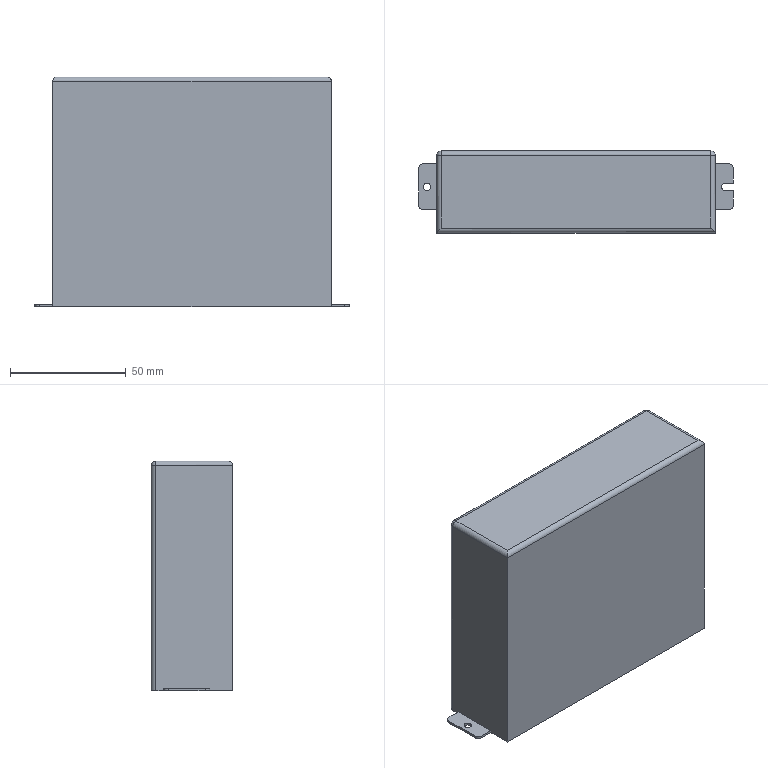Part | NX | features BREP 1 | 1 solid | 31 faces | box 136 x 35.4 x 99.5 mm | volume 424636 mm3 | plane 17 | cylinder 12 | sphere 2 | commonest cylinder face diameters 4 x10 3.2 x2
STEP:
#1=CARTESIAN_POINT('',(-66.1,2.3,0.));
#2=VERTEX_POINT('',#1);
#3=CARTESIAN_POINT('',(-64.5,2.3,0.));
#4=DIRECTION('',(0.,0.,-1.));
#5=DIRECTION('',(-1.,0.,0.));
#6=AXIS2_PLACEMENT_3D('',#3,#4,#5);
#7=CIRCLE('',#6,1.6);
#8=EDGE_CURVE('',#2,#2,#7,.T.);
#9=ORIENTED_EDGE('',*,*,#8,.T.);
#10=EDGE_LOOP('',(#9));
#11=FACE_BOUND('',#10,.T.);
#12=CARTESIAN_POINT('',(-66.1,2.3,1.));
#13=VERTEX_POINT('',#12);
#14=CARTESIAN_POINT('',(-64.5,2.3,1.));
#15=DIRECTION('',(0.,0.,-1.));
#16=DIRECTION('',(-1.,0.,0.));
#17=AXIS2_PLACEMENT_3D('',#14,#15,#16);
#18=CIRCLE('',#17,1.6);
#19=EDGE_CURVE('',#13,#13,#18,.T.);
#20=ORIENTED_EDGE('',*,*,#19,.F.);
#21=EDGE_LOOP('',(#20));
#22=FACE_BOUND('',#21,.T.);
#23=CARTESIAN_POINT('',(-64.5,2.3,10.));
#24=DIRECTION('',(0.,0.,-1.));
#25=DIRECTION('',(-1.,0.,0.));
#26=AXIS2_PLACEMENT_3D('',#23,#24,#25);
#27=CYLINDRICAL_SURFACE('',#26,1.6);
#28=ADVANCED_FACE('',(#11,#22),#27,.F.);
#29=CARTESIAN_POINT('',(64.5,3.9,1.));
#30=VERTEX_POINT('',#29);
#31=CARTESIAN_POINT('',(64.5,0.7,1.));
#32=VERTEX_POINT('',#31);
#33=CARTESIAN_POINT('',(64.5,2.3,1.));
#34=DIRECTION('',(0.,0.,1.));
#35=DIRECTION('',(1.,0.,0.));
#36=AXIS2_PLACEMENT_3D('',#33,#34,#35);
#37=CIRCLE('',#36,1.6);
#38=EDGE_CURVE('',#30,#32,#37,.T.);
#39=ORIENTED_EDGE('',*,*,#38,.T.);
#40=CARTESIAN_POINT('',(64.5,0.7,0.));
#41=VERTEX_POINT('',#40);
#42=CARTESIAN_POINT('',(64.5,0.7,10.));
#43=DIRECTION('',(0.,0.,-1.));
#44=VECTOR('',#43,1000.);
#45=LINE('',#42,#44);
#46=EDGE_CURVE('',#32,#41,#45,.T.);
#47=ORIENTED_EDGE('',*,*,#46,.T.);
#48=CARTESIAN_POINT('',(64.5,3.9,0.));
#49=VERTEX_POINT('',#48);
#50=CARTESIAN_POINT('',(64.5,2.3,0.));
#51=DIRECTION('',(0.,0.,-1.));
#52=DIRECTION('',(-1.,0.,0.));
#53=AXIS2_PLACEMENT_3D('',#50,#51,#52);
#54=CIRCLE('',#53,1.6);
#55=EDGE_CURVE('',#41,#49,#54,.T.);
#56=ORIENTED_EDGE('',*,*,#55,.T.);
#57=CARTESIAN_POINT('',(64.5,3.9,10.));
#58=DIRECTION('',(0.,0.,-1.));
#59=VECTOR('',#58,1000.);
#60=LINE('',#57,#59);
#61=EDGE_CURVE('',#30,#49,#60,.T.);
#62=ORIENTED_EDGE('',*,*,#61,.F.);
#63=EDGE_LOOP('',(#39,#47,#56,#62));
#64=FACE_BOUND('',#63,.T.);
#65=CARTESIAN_POINT('',(64.5,2.3,10.));
#66=DIRECTION('',(0.,0.,-1.));
#67=DIRECTION('',(-1.,0.,0.));
#68=AXIS2_PLACEMENT_3D('',#65,#66,#67);
#69=CYLINDRICAL_SURFACE('',#68,1.6);
#70=ADVANCED_FACE('',(#64),#69,.F.);
#71=CARTESIAN_POINT('',(68.,0.7,1.));
#72=VERTEX_POINT('',#71);
#73=CARTESIAN_POINT('',(68.,0.7,0.));
#74=VERTEX_POINT('',#73);
#75=CARTESIAN_POINT('',(68.,0.7,10.));
#76=DIRECTION('',(0.,0.,-1.));
#77=VECTOR('',#76,1000.);
#78=LINE('',#75,#77);
#79=EDGE_CURVE('',#72,#74,#78,.T.);
#80=ORIENTED_EDGE('',*,*,#79,.F.);
#81=CARTESIAN_POINT('',(68.,-5.7,1.));
#82=VERTEX_POINT('',#81);
#83=CARTESIAN_POINT('',(68.,0.05,1.));
#84=DIRECTION('',(0.,-1.,0.));
#85=VECTOR('',#84,1000.);
#86=LINE('',#83,#85);
#87=EDGE_CURVE('',#72,#82,#86,.T.);
#88=ORIENTED_EDGE('',*,*,#87,.T.);
#89=CARTESIAN_POINT('',(68.,-5.7,0.));
#90=VERTEX_POINT('',#89);
#91=CARTESIAN_POINT('',(68.,-5.7,1.));
#92=DIRECTION('',(0.,0.,-1.));
#93=VECTOR('',#92,1000.);
#94=LINE('',#91,#93);
#95=EDGE_CURVE('',#82,#90,#94,.T.);
#96=ORIENTED_EDGE('',*,*,#95,.T.);
#97=CARTESIAN_POINT('',(68.,10.3,0.));
#98=DIRECTION('',(0.,-1.,0.));
#99=VECTOR('',#98,1000.);
#100=LINE('',#97,#99);
#101=EDGE_CURVE('',#74,#90,#100,.T.);
#102=ORIENTED_EDGE('',*,*,#101,.F.);
#103=EDGE_LOOP('',(#80,#88,#96,#102));
#104=FACE_BOUND('',#103,.T.);
#105=CARTESIAN_POINT('',(68.,0.05,1.));
#106=DIRECTION('',(1.,0.,0.));
#107=DIRECTION('',(0.,1.,0.));
#108=AXIS2_PLACEMENT_3D('',#105,#106,#107);
#109=PLANE('',#108);
#110=ADVANCED_FACE('',(#104),#109,.T.);
#111=ORIENTED_EDGE('',*,*,#19,.T.);
#112=EDGE_LOOP('',(#111));
#113=FACE_BOUND('',#112,.T.);
#114=CARTESIAN_POINT('',(-68.,10.3,1.));
#115=VERTEX_POINT('',#114);
#116=CARTESIAN_POINT('',(-66.,12.3,1.));
#117=VERTEX_POINT('',#116);
#118=CARTESIAN_POINT('',(-66.,10.3,1.));
#119=DIRECTION('',(0.,0.,-1.));
#120=DIRECTION('',(-1.,0.,0.));
#121=AXIS2_PLACEMENT_3D('',#118,#119,#120);
#122=CIRCLE('',#121,2.);
#123=EDGE_CURVE('',#115,#117,#122,.T.);
#124=ORIENTED_EDGE('',*,*,#123,.F.);
#125=CARTESIAN_POINT('',(-68.,-5.7,1.));
#126=VERTEX_POINT('',#125);
#127=CARTESIAN_POINT('',(-68.,-1.725,1.));
#128=DIRECTION('',(0.,1.,0.));
#129=VECTOR('',#128,1000.);
#130=LINE('',#127,#129);
#131=EDGE_CURVE('',#126,#115,#130,.T.);
#132=ORIENTED_EDGE('',*,*,#131,.F.);
#133=CARTESIAN_POINT('',(-66.,-7.7,1.));
#134=VERTEX_POINT('',#133);
#135=CARTESIAN_POINT('',(-66.,-5.7,1.));
#136=DIRECTION('',(0.,0.,-1.));
#137=DIRECTION('',(-1.,0.,0.));
#138=AXIS2_PLACEMENT_3D('',#135,#136,#137);
#139=CIRCLE('',#138,2.);
#140=EDGE_CURVE('',#134,#126,#139,.T.);
#141=ORIENTED_EDGE('',*,*,#140,.F.);
#142=CARTESIAN_POINT('',(-60.3,-7.7,1.));
#143=VERTEX_POINT('',#142);
#144=CARTESIAN_POINT('',(-66.,-7.7,1.));
#145=DIRECTION('',(-1.,0.,0.));
#146=VECTOR('',#145,1000.);
#147=LINE('',#144,#146);
#148=EDGE_CURVE('',#143,#134,#147,.T.);
#149=ORIENTED_EDGE('',*,*,#148,.F.);
#150=CARTESIAN_POINT('',(-60.3,12.3,1.));
#151=VERTEX_POINT('',#150);
#152=CARTESIAN_POINT('',(-60.3,12.3,1.));
#153=DIRECTION('',(0.,-1.,0.));
#154=VECTOR('',#153,1000.);
#155=LINE('',#152,#154);
#156=EDGE_CURVE('',#151,#143,#155,.T.);
#157=ORIENTED_EDGE('',*,*,#156,.F.);
#158=CARTESIAN_POINT('',(-60.3,12.3,1.));
#159=DIRECTION('',(1.,0.,0.));
#160=VECTOR('',#159,1000.);
#161=LINE('',#158,#160);
#162=EDGE_CURVE('',#117,#151,#161,.T.);
#163=ORIENTED_EDGE('',*,*,#162,.F.);
#164=EDGE_LOOP('',(#124,#132,#141,#149,#157,#163));
#165=FACE_BOUND('',#164,.T.);
#166=CARTESIAN_POINT('',(-66.,10.3,1.));
#167=DIRECTION('',(0.,0.,-1.));
#168=DIRECTION('',(0.,-1.,0.));
#169=AXIS2_PLACEMENT_3D('',#166,#167,#168);
#170=PLANE('',#169);
#171=ADVANCED_FACE('',(#113,#165),#170,.F.);
#172=CARTESIAN_POINT('',(-66.,12.3,0.));
#173=VERTEX_POINT('',#172);
#174=CARTESIAN_POINT('',(-60.3,12.3,0.));
#175=VERTEX_POINT('',#174);
#176=CARTESIAN_POINT('',(-60.3,12.3,0.));
#177=DIRECTION('',(1.,0.,0.));
#178=VECTOR('',#177,1000.);
#179=LINE('',#176,#178);
#180=EDGE_CURVE('',#173,#175,#179,.T.);
#181=ORIENTED_EDGE('',*,*,#180,.F.);
#182=CARTESIAN_POINT('',(-66.,12.3,1.));
#183=DIRECTION('',(0.,0.,-1.));
#184=VECTOR('',#183,1000.);
#185=LINE('',#182,#184);
#186=EDGE_CURVE('',#117,#173,#185,.T.);
#187=ORIENTED_EDGE('',*,*,#186,.F.);
#188=ORIENTED_EDGE('',*,*,#162,.T.);
#189=CARTESIAN_POINT('',(-60.3,12.3,1.));
#190=DIRECTION('',(0.,0.,-1.));
#191=VECTOR('',#190,1000.);
#192=LINE('',#189,#191);
#193=EDGE_CURVE('',#151,#175,#192,.T.);
#194=ORIENTED_EDGE('',*,*,#193,.T.);
#195=EDGE_LOOP('',(#181,#187,#188,#194));
#196=FACE_BOUND('',#195,.T.);
#197=CARTESIAN_POINT('',(-60.3,12.3,1.));
#198=DIRECTION('',(0.,1.,0.));
#199=DIRECTION('',(1.,0.,0.));
#200=AXIS2_PLACEMENT_3D('',#197,#198,#199);
#201=PLANE('',#200);
#202=ADVANCED_FACE('',(#196),#201,.T.);
#203=CARTESIAN_POINT('',(-60.3,-7.7,0.));
#204=VERTEX_POINT('',#203);
#205=CARTESIAN_POINT('',(-66.,-7.7,0.));
#206=VERTEX_POINT('',#205);
#207=CARTESIAN_POINT('',(-66.,-7.7,0.));
#208=DIRECTION('',(-1.,0.,0.));
#209=VECTOR('',#208,1000.);
#210=LINE('',#207,#209);
#211=EDGE_CURVE('',#204,#206,#210,.T.);
#212=ORIENTED_EDGE('',*,*,#211,.F.);
#213=CARTESIAN_POINT('',(-60.3,-7.7,1.));
#214=DIRECTION('',(0.,0.,-1.));
#215=VECTOR('',#214,1000.);
#216=LINE('',#213,#215);
#217=EDGE_CURVE('',#143,#204,#216,.T.);
#218=ORIENTED_EDGE('',*,*,#217,.F.);
#219=ORIENTED_EDGE('',*,*,#148,.T.);
#220=CARTESIAN_POINT('',(-66.,-7.7,1.));
#221=DIRECTION('',(0.,0.,-1.));
#222=VECTOR('',#221,1000.);
#223=LINE('',#220,#222);
#224=EDGE_CURVE('',#134,#206,#223,.T.);
#225=ORIENTED_EDGE('',*,*,#224,.T.);
#226=EDGE_LOOP('',(#212,#218,#219,#225));
#227=FACE_BOUND('',#226,.T.);
#228=CARTESIAN_POINT('',(-66.,-7.7,1.));
#229=DIRECTION('',(0.,-1.,0.));
#230=DIRECTION('',(0.,0.,-1.));
#231=AXIS2_PLACEMENT_3D('',#228,#229,#230);
#232=PLANE('',#231);
#233=ADVANCED_FACE('',(#227),#232,.T.);
#234=CARTESIAN_POINT('',(-68.,-5.7,0.));
#235=VERTEX_POINT('',#234);
#236=CARTESIAN_POINT('',(-66.,-5.7,0.));
#237=DIRECTION('',(0.,0.,-1.));
#238=DIRECTION('',(-1.,0.,0.));
#239=AXIS2_PLACEMENT_3D('',#236,#237,#238);
#240=CIRCLE('',#239,2.);
#241=EDGE_CURVE('',#206,#235,#240,.T.);
#242=ORIENTED_EDGE('',*,*,#241,.F.);
#243=ORIENTED_EDGE('',*,*,#224,.F.);
#244=ORIENTED_EDGE('',*,*,#140,.T.);
#245=CARTESIAN_POINT('',(-68.,-5.7,1.));
#246=DIRECTION('',(0.,0.,-1.));
#247=VECTOR('',#246,1000.);
#248=LINE('',#245,#247);
#249=EDGE_CURVE('',#126,#235,#248,.T.);
#250=ORIENTED_EDGE('',*,*,#249,.T.);
#251=EDGE_LOOP('',(#242,#243,#244,#250));
#252=FACE_BOUND('',#251,.T.);
#253=CARTESIAN_POINT('',(-66.,-5.7,1.));
#254=DIRECTION('',(0.,0.,-1.));
#255=DIRECTION('',(-1.,0.,0.));
#256=AXIS2_PLACEMENT_3D('',#253,#254,#255);
#257=CYLINDRICAL_SURFACE('',#256,2.);
#258=ADVANCED_FACE('',(#252),#257,.T.);
#259=CARTESIAN_POINT('',(-68.,10.3,0.));
#260=VERTEX_POINT('',#259);
#261=CARTESIAN_POINT('',(-68.,10.3,0.));
#262=DIRECTION('',(0.,1.,0.));
#263=VECTOR('',#262,1000.);
#264=LINE('',#261,#263);
#265=EDGE_CURVE('',#235,#260,#264,.T.);
#266=ORIENTED_EDGE('',*,*,#265,.F.);
#267=ORIENTED_EDGE('',*,*,#249,.F.);
#268=ORIENTED_EDGE('',*,*,#131,.T.);
#269=CARTESIAN_POINT('',(-68.,10.3,1.));
#270=DIRECTION('',(0.,0.,-1.));
#271=VECTOR('',#270,1000.);
#272=LINE('',#269,#271);
#273=EDGE_CURVE('',#115,#260,#272,.T.);
#274=ORIENTED_EDGE('',*,*,#273,.T.);
#275=EDGE_LOOP('',(#266,#267,#268,#274));
#276=FACE_BOUND('',#275,.T.);
#277=CARTESIAN_POINT('',(-68.,10.3,1.));
#278=DIRECTION('',(-1.,0.,0.));
#279=DIRECTION('',(0.,0.,1.));
#280=AXIS2_PLACEMENT_3D('',#277,#278,#279);
#281=PLANE('',#280);
#282=ADVANCED_FACE('',(#276),#281,.T.);
#283=CARTESIAN_POINT('',(-66.,10.3,0.));
#284=DIRECTION('',(0.,0.,-1.));
#285=DIRECTION('',(-1.,0.,0.));
#286=AXIS2_PLACEMENT_3D('',#283,#284,#285);
#287=CIRCLE('',#286,2.);
#288=EDGE_CURVE('',#260,#173,#287,.T.);
#289=ORIENTED_EDGE('',*,*,#288,.F.);
#290=ORIENTED_EDGE('',*,*,#273,.F.);
#291=ORIENTED_EDGE('',*,*,#123,.T.);
#292=ORIENTED_EDGE('',*,*,#186,.T.);
#293=EDGE_LOOP('',(#289,#290,#291,#292));
#294=FACE_BOUND('',#293,.T.);
#295=CARTESIAN_POINT('',(-66.,10.3,1.));
#296=DIRECTION('',(0.,0.,-1.));
#297=DIRECTION('',(-1.,0.,0.));
#298=AXIS2_PLACEMENT_3D('',#295,#296,#297);
#299=CYLINDRICAL_SURFACE('',#298,2.);
#300=ADVANCED_FACE('',(#294),#299,.T.);
#301=CARTESIAN_POINT('',(66.,0.7,1.));
#302=DIRECTION('',(1.,0.,0.));
#303=VECTOR('',#302,1000.);
#304=LINE('',#301,#303);
#305=EDGE_CURVE('',#32,#72,#304,.T.);
#306=ORIENTED_EDGE('',*,*,#305,.F.);
#307=ORIENTED_EDGE('',*,*,#38,.F.);
#308=CARTESIAN_POINT('',(68.,3.9,1.));
#309=VERTEX_POINT('',#308);
#310=CARTESIAN_POINT('',(66.,3.9,1.));
#311=DIRECTION('',(-1.,0.,0.));
#312=VECTOR('',#311,1000.);
#313=LINE('',#310,#312);
#314=EDGE_CURVE('',#309,#30,#313,.T.);
#315=ORIENTED_EDGE('',*,*,#314,.F.);
#316=CARTESIAN_POINT('',(68.,10.3,1.));
#317=VERTEX_POINT('',#316);
#318=CARTESIAN_POINT('',(68.,0.05,1.));
#319=DIRECTION('',(0.,-1.,0.));
#320=VECTOR('',#319,1000.);
#321=LINE('',#318,#320);
#322=EDGE_CURVE('',#317,#309,#321,.T.);
#323=ORIENTED_EDGE('',*,*,#322,.F.);
#324=CARTESIAN_POINT('',(66.,12.3,1.));
#325=VERTEX_POINT('',#324);
#326=CARTESIAN_POINT('',(66.,10.3,1.));
#327=DIRECTION('',(0.,0.,-1.));
#328=DIRECTION('',(1.,0.,0.));
#329=AXIS2_PLACEMENT_3D('',#326,#327,#328);
#330=CIRCLE('',#329,2.);
#331=EDGE_CURVE('',#325,#317,#330,.T.);
#332=ORIENTED_EDGE('',*,*,#331,.F.);
#333=CARTESIAN_POINT('',(60.3,12.3,1.));
#334=VERTEX_POINT('',#333);
#335=CARTESIAN_POINT('',(60.3,12.3,1.));
#336=DIRECTION('',(1.,0.,0.));
#337=VECTOR('',#336,1000.);
#338=LINE('',#335,#337);
#339=EDGE_CURVE('',#334,#325,#338,.T.);
#340=ORIENTED_EDGE('',*,*,#339,.F.);
#341=CARTESIAN_POINT('',(60.3,-7.7,1.));
#342=VERTEX_POINT('',#341);
#343=CARTESIAN_POINT('',(60.3,12.3,1.));
#344=DIRECTION('',(0.,1.,0.));
#345=VECTOR('',#344,1000.);
#346=LINE('',#343,#345);
#347=EDGE_CURVE('',#342,#334,#346,.T.);
#348=ORIENTED_EDGE('',*,*,#347,.F.);
#349=CARTESIAN_POINT('',(66.,-7.7,1.));
#350=VERTEX_POINT('',#349);
#351=CARTESIAN_POINT('',(66.,-7.7,1.));
#352=DIRECTION('',(-1.,0.,0.));
#353=VECTOR('',#352,1000.);
#354=LINE('',#351,#353);
#355=EDGE_CURVE('',#350,#342,#354,.T.);
#356=ORIENTED_EDGE('',*,*,#355,.F.);
#357=CARTESIAN_POINT('',(66.,-5.7,1.));
#358=DIRECTION('',(0.,0.,-1.));
#359=DIRECTION('',(1.,0.,0.));
#360=AXIS2_PLACEMENT_3D('',#357,#358,#359);
#361=CIRCLE('',#360,2.);
#362=EDGE_CURVE('',#82,#350,#361,.T.);
#363=ORIENTED_EDGE('',*,*,#362,.F.);
#364=ORIENTED_EDGE('',*,*,#87,.F.);
#365=EDGE_LOOP('',(#306,#307,#315,#323,#332,#340,#348,#356,#363,#364));
#366=FACE_BOUND('',#365,.T.);
#367=CARTESIAN_POINT('',(66.,-5.7,1.));
#368=DIRECTION('',(0.,0.,1.));
#369=DIRECTION('',(1.,0.,0.));
#370=AXIS2_PLACEMENT_3D('',#367,#368,#369);
#371=PLANE('',#370);
#372=ADVANCED_FACE('',(#366),#371,.T.);
#373=CARTESIAN_POINT('',(60.3,12.3,0.));
#374=VERTEX_POINT('',#373);
#375=CARTESIAN_POINT('',(66.,12.3,0.));
#376=VERTEX_POINT('',#375);
#377=CARTESIAN_POINT('',(60.3,12.3,0.));
#378=DIRECTION('',(1.,0.,0.));
#379=VECTOR('',#378,1000.);
#380=LINE('',#377,#379);
#381=EDGE_CURVE('',#374,#376,#380,.T.);
#382=ORIENTED_EDGE('',*,*,#381,.F.);
#383=CARTESIAN_POINT('',(60.3,12.3,1.));
#384=DIRECTION('',(0.,0.,-1.));
#385=VECTOR('',#384,1000.);
#386=LINE('',#383,#385);
#387=EDGE_CURVE('',#334,#374,#386,.T.);
#388=ORIENTED_EDGE('',*,*,#387,.F.);
#389=ORIENTED_EDGE('',*,*,#339,.T.);
#390=CARTESIAN_POINT('',(66.,12.3,1.));
#391=DIRECTION('',(0.,0.,-1.));
#392=VECTOR('',#391,1000.);
#393=LINE('',#390,#392);
#394=EDGE_CURVE('',#325,#376,#393,.T.);
#395=ORIENTED_EDGE('',*,*,#394,.T.);
#396=EDGE_LOOP('',(#382,#388,#389,#395));
#397=FACE_BOUND('',#396,.T.);
#398=CARTESIAN_POINT('',(60.3,12.3,1.));
#399=DIRECTION('',(0.,1.,0.));
#400=DIRECTION('',(1.,0.,0.));
#401=AXIS2_PLACEMENT_3D('',#398,#399,#400);
#402=PLANE('',#401);
#403=ADVANCED_FACE('',(#397),#402,.T.);
#404=CARTESIAN_POINT('',(68.,10.3,0.));
#405=VERTEX_POINT('',#404);
#406=CARTESIAN_POINT('',(66.,10.3,0.));
#407=DIRECTION('',(0.,0.,-1.));
#408=DIRECTION('',(1.,0.,0.));
#409=AXIS2_PLACEMENT_3D('',#406,#407,#408);
#410=CIRCLE('',#409,2.);
#411=EDGE_CURVE('',#376,#405,#410,.T.);
#412=ORIENTED_EDGE('',*,*,#411,.F.);
#413=ORIENTED_EDGE('',*,*,#394,.F.);
#414=ORIENTED_EDGE('',*,*,#331,.T.);
#415=CARTESIAN_POINT('',(68.,10.3,1.));
#416=DIRECTION('',(0.,0.,-1.));
#417=VECTOR('',#416,1000.);
#418=LINE('',#415,#417);
#419=EDGE_CURVE('',#317,#405,#418,.T.);
#420=ORIENTED_EDGE('',*,*,#419,.T.);
#421=EDGE_LOOP('',(#412,#413,#414,#420));
#422=FACE_BOUND('',#421,.T.);
#423=CARTESIAN_POINT('',(66.,10.3,1.));
#424=DIRECTION('',(0.,0.,-1.));
#425=DIRECTION('',(-1.,0.,0.));
#426=AXIS2_PLACEMENT_3D('',#423,#424,#425);
#427=CYLINDRICAL_SURFACE('',#426,2.);
#428=ADVANCED_FACE('',(#422),#427,.T.);
#429=CARTESIAN_POINT('',(68.,3.9,0.));
#430=VERTEX_POINT('',#429);
#431=CARTESIAN_POINT('',(68.,3.9,10.));
#432=DIRECTION('',(0.,0.,-1.));
#433=VECTOR('',#432,1000.);
#434=LINE('',#431,#433);
#435=EDGE_CURVE('',#309,#430,#434,.T.);
#436=ORIENTED_EDGE('',*,*,#435,.T.);
#437=CARTESIAN_POINT('',(68.,10.3,0.));
#438=DIRECTION('',(0.,-1.,0.));
#439=VECTOR('',#438,1000.);
#440=LINE('',#437,#439);
#441=EDGE_CURVE('',#405,#430,#440,.T.);
#442=ORIENTED_EDGE('',*,*,#441,.F.);
#443=ORIENTED_EDGE('',*,*,#419,.F.);
#444=ORIENTED_EDGE('',*,*,#322,.T.);
#445=EDGE_LOOP('',(#436,#442,#443,#444));
#446=FACE_BOUND('',#445,.T.);
#447=CARTESIAN_POINT('',(68.,0.05,1.));
#448=DIRECTION('',(1.,0.,0.));
#449=DIRECTION('',(0.,1.,0.));
#450=AXIS2_PLACEMENT_3D('',#447,#448,#449);
#451=PLANE('',#450);
#452=ADVANCED_FACE('',(#446),#451,.T.);
#453=CARTESIAN_POINT('',(66.,-7.7,0.));
#454=VERTEX_POINT('',#453);
#455=CARTESIAN_POINT('',(66.,-5.7,0.));
#456=DIRECTION('',(0.,0.,-1.));
#457=DIRECTION('',(1.,0.,0.));
#458=AXIS2_PLACEMENT_3D('',#455,#456,#457);
#459=CIRCLE('',#458,2.);
#460=EDGE_CURVE('',#90,#454,#459,.T.);
#461=ORIENTED_EDGE('',*,*,#460,.F.);
#462=ORIENTED_EDGE('',*,*,#95,.F.);
#463=ORIENTED_EDGE('',*,*,#362,.T.);
#464=CARTESIAN_POINT('',(66.,-7.7,1.));
#465=DIRECTION('',(0.,0.,-1.));
#466=VECTOR('',#465,1000.);
#467=LINE('',#464,#466);
#468=EDGE_CURVE('',#350,#454,#467,.T.);
#469=ORIENTED_EDGE('',*,*,#468,.T.);
#470=EDGE_LOOP('',(#461,#462,#463,#469));
#471=FACE_BOUND('',#470,.T.);
#472=CARTESIAN_POINT('',(66.,-5.7,1.));
#473=DIRECTION('',(0.,0.,-1.));
#474=DIRECTION('',(-1.,0.,0.));
#475=AXIS2_PLACEMENT_3D('',#472,#473,#474);
#476=CYLINDRICAL_SURFACE('',#475,2.);
#477=ADVANCED_FACE('',(#471),#476,.T.);
#478=CARTESIAN_POINT('',(60.3,-7.7,0.));
#479=VERTEX_POINT('',#478);
#480=CARTESIAN_POINT('',(66.,-7.7,0.));
#481=DIRECTION('',(-1.,0.,0.));
#482=VECTOR('',#481,1000.);
#483=LINE('',#480,#482);
#484=EDGE_CURVE('',#454,#479,#483,.T.);
#485=ORIENTED_EDGE('',*,*,#484,.F.);
#486=ORIENTED_EDGE('',*,*,#468,.F.);
#487=ORIENTED_EDGE('',*,*,#355,.T.);
#488=CARTESIAN_POINT('',(60.3,-7.7,1.));
#489=DIRECTION('',(0.,0.,-1.));
#490=VECTOR('',#489,1000.);
#491=LINE('',#488,#490);
#492=EDGE_CURVE('',#342,#479,#491,.T.);
#493=ORIENTED_EDGE('',*,*,#492,.T.);
#494=EDGE_LOOP('',(#485,#486,#487,#493));
#495=FACE_BOUND('',#494,.T.);
#496=CARTESIAN_POINT('',(66.,-7.7,1.));
#497=DIRECTION('',(0.,-1.,0.));
#498=DIRECTION('',(0.,0.,-1.));
#499=AXIS2_PLACEMENT_3D('',#496,#497,#498);
#500=PLANE('',#499);
#501=ADVANCED_FACE('',(#495),#500,.T.);
#502=CARTESIAN_POINT('',(-58.3,-15.7,99.5));
#503=VERTEX_POINT('',#502);
#504=CARTESIAN_POINT('',(-60.3,-17.7,97.5));
#505=VERTEX_POINT('',#504);
#506=CARTESIAN_POINT('',(-58.3,-15.7,99.5));
#507=CARTESIAN_POINT('',(-59.472,-16.872,99.5));
#508=CARTESIAN_POINT('',(-60.3,-17.7,98.672));
#509=CARTESIAN_POINT('',(-60.3,-17.7,97.5));
#510=(BOUNDED_CURVE()B_SPLINE_CURVE(3,(#506,#507,#508,#509),.UNSPECIFIED.,.F.,.F.)B_SPLINE_CURVE_WITH_KNOTS((4,4),(0.,1.),.PIECEWISE_BEZIER_KNOTS.)CURVE()GEOMETRIC_REPRESENTATION_ITEM()RATIONAL_B_SPLINE_CURVE((1.,0.8047,0.8047,1.))REPRESENTATION_ITEM(''));
#511=EDGE_CURVE('',#503,#505,#510,.T.);
#512=ORIENTED_EDGE('',*,*,#511,.T.);
#513=CARTESIAN_POINT('',(60.3,-17.7,97.5));
#514=VERTEX_POINT('',#513);
#515=CARTESIAN_POINT('',(-60.3,-17.7,97.5));
#516=DIRECTION('',(-1.,0.,0.));
#517=VECTOR('',#516,1000.);
#518=LINE('',#515,#517);
#519=EDGE_CURVE('',#514,#505,#518,.T.);
#520=ORIENTED_EDGE('',*,*,#519,.F.);
#521=CARTESIAN_POINT('',(58.3,-15.7,99.5));
#522=VERTEX_POINT('',#521);
#523=CARTESIAN_POINT('',(60.3,-17.7,97.5));
#524=CARTESIAN_POINT('',(60.3,-17.7,98.672));
#525=CARTESIAN_POINT('',(59.472,-16.872,99.5));
#526=CARTESIAN_POINT('',(58.3,-15.7,99.5));
#527=(BOUNDED_CURVE()B_SPLINE_CURVE(3,(#523,#524,#525,#526),.UNSPECIFIED.,.F.,.F.)B_SPLINE_CURVE_WITH_KNOTS((4,4),(0.,1.),.PIECEWISE_BEZIER_KNOTS.)CURVE()GEOMETRIC_REPRESENTATION_ITEM()RATIONAL_B_SPLINE_CURVE((1.,0.8047,0.8047,1.))REPRESENTATION_ITEM(''));
#528=EDGE_CURVE('',#514,#522,#527,.T.);
#529=ORIENTED_EDGE('',*,*,#528,.T.);
#530=CARTESIAN_POINT('',(60.3,-15.7,99.5));
#531=DIRECTION('',(1.,0.,0.));
#532=VECTOR('',#531,1000.);
#533=LINE('',#530,#532);
#534=EDGE_CURVE('',#503,#522,#533,.T.);
#535=ORIENTED_EDGE('',*,*,#534,.F.);
#536=EDGE_LOOP('',(#512,#520,#529,#535));
#537=FACE_BOUND('',#536,.T.);
#538=CARTESIAN_POINT('',(0.,-15.7,97.5));
#539=DIRECTION('',(-1.,0.,0.));
#540=DIRECTION('',(0.,0.,1.));
#541=AXIS2_PLACEMENT_3D('',#538,#539,#540);
#542=CYLINDRICAL_SURFACE('',#541,2.);
#543=ADVANCED_FACE('',(#537),#542,.T.);
#544=CARTESIAN_POINT('',(60.3,15.7,97.5));
#545=VERTEX_POINT('',#544);
#546=CARTESIAN_POINT('',(58.3,15.7,99.5));
#547=VERTEX_POINT('',#546);
#548=CARTESIAN_POINT('',(58.3,15.7,97.5));
#549=DIRECTION('',(0.,-1.,0.));
#550=DIRECTION('',(0.,0.,1.));
#551=AXIS2_PLACEMENT_3D('',#548,#549,#550);
#552=CIRCLE('',#551,2.);
#553=EDGE_CURVE('',#545,#547,#552,.T.);
#554=ORIENTED_EDGE('',*,*,#553,.T.);
#555=CARTESIAN_POINT('',(58.3,17.7,99.5));
#556=DIRECTION('',(0.,1.,0.));
#557=VECTOR('',#556,1000.);
#558=LINE('',#555,#557);
#559=EDGE_CURVE('',#522,#547,#558,.T.);
#560=ORIENTED_EDGE('',*,*,#559,.F.);
#561=ORIENTED_EDGE('',*,*,#528,.F.);
#562=CARTESIAN_POINT('',(60.3,-17.7,97.5));
#563=DIRECTION('',(0.,-1.,0.));
#564=VECTOR('',#563,1000.);
#565=LINE('',#562,#564);
#566=EDGE_CURVE('',#545,#514,#565,.T.);
#567=ORIENTED_EDGE('',*,*,#566,.F.);
#568=EDGE_LOOP('',(#554,#560,#561,#567));
#569=FACE_BOUND('',#568,.T.);
#570=CARTESIAN_POINT('',(58.3,0.,97.5));
#571=DIRECTION('',(0.,-1.,0.));
#572=DIRECTION('',(0.,0.,-1.));
#573=AXIS2_PLACEMENT_3D('',#570,#571,#572);
#574=CYLINDRICAL_SURFACE('',#573,2.);
#575=ADVANCED_FACE('',(#569),#574,.T.);
#576=CARTESIAN_POINT('',(-58.3,15.7,99.5));
#577=VERTEX_POINT('',#576);
#578=CARTESIAN_POINT('',(-60.3,15.7,97.5));
#579=VERTEX_POINT('',#578);
#580=CARTESIAN_POINT('',(-58.3,15.7,97.5));
#581=DIRECTION('',(0.,-1.,0.));
#582=DIRECTION('',(0.,0.,1.));
#583=AXIS2_PLACEMENT_3D('',#580,#581,#582);
#584=CIRCLE('',#583,2.);
#585=EDGE_CURVE('',#577,#579,#584,.T.);
#586=ORIENTED_EDGE('',*,*,#585,.T.);
#587=CARTESIAN_POINT('',(-60.3,17.7,97.5));
#588=DIRECTION('',(0.,1.,0.));
#589=VECTOR('',#588,1000.);
#590=LINE('',#587,#589);
#591=EDGE_CURVE('',#505,#579,#590,.T.);
#592=ORIENTED_EDGE('',*,*,#591,.F.);
#593=ORIENTED_EDGE('',*,*,#511,.F.);
#594=CARTESIAN_POINT('',(-58.3,-17.7,99.5));
#595=DIRECTION('',(0.,-1.,0.));
#596=VECTOR('',#595,1000.);
#597=LINE('',#594,#596);
#598=EDGE_CURVE('',#577,#503,#597,.T.);
#599=ORIENTED_EDGE('',*,*,#598,.F.);
#600=EDGE_LOOP('',(#586,#592,#593,#599));
#601=FACE_BOUND('',#600,.T.);
#602=CARTESIAN_POINT('',(-58.3,0.,97.5));
#603=DIRECTION('',(0.,1.,0.));
#604=DIRECTION('',(0.,0.,1.));
#605=AXIS2_PLACEMENT_3D('',#602,#603,#604);
#606=CYLINDRICAL_SURFACE('',#605,2.);
#607=ADVANCED_FACE('',(#601),#606,.T.);
#608=CARTESIAN_POINT('',(58.3,17.7,97.5));
#609=VERTEX_POINT('',#608);
#610=CARTESIAN_POINT('',(58.3,15.7,97.5));
#611=DIRECTION('',(0.,0.,1.));
#612=DIRECTION('',(1.,0.,0.));
#613=AXIS2_PLACEMENT_3D('',#610,#611,#612);
#614=CIRCLE('',#613,2.);
#615=EDGE_CURVE('',#545,#609,#614,.T.);
#616=ORIENTED_EDGE('',*,*,#615,.T.);
#617=CARTESIAN_POINT('',(58.3,15.7,97.5));
#618=DIRECTION('',(1.,0.,0.));
#619=DIRECTION('',(0.,0.,-1.));
#620=AXIS2_PLACEMENT_3D('',#617,#618,#619);
#621=CIRCLE('',#620,2.);
#622=EDGE_CURVE('',#609,#547,#621,.T.);
#623=ORIENTED_EDGE('',*,*,#622,.T.);
#624=ORIENTED_EDGE('',*,*,#553,.F.);
#625=EDGE_LOOP('',(#616,#623,#624));
#626=FACE_BOUND('',#625,.T.);
#627=CARTESIAN_POINT('',(58.3,15.7,97.5));
#628=DIRECTION('',(0.,0.,-1.));
#629=DIRECTION('',(1.,0.,0.));
#630=AXIS2_PLACEMENT_3D('',#627,#628,#629);
#631=SPHERICAL_SURFACE('',#630,2.);
#632=ADVANCED_FACE('',(#626),#631,.T.);
#633=CARTESIAN_POINT('',(-58.3,17.7,97.5));
#634=VERTEX_POINT('',#633);
#635=CARTESIAN_POINT('',(-58.3,15.7,97.5));
#636=DIRECTION('',(-1.,0.,0.));
#637=DIRECTION('',(0.,0.,1.));
#638=AXIS2_PLACEMENT_3D('',#635,#636,#637);
#639=CIRCLE('',#638,2.);
#640=EDGE_CURVE('',#577,#634,#639,.T.);
#641=ORIENTED_EDGE('',*,*,#640,.T.);
#642=CARTESIAN_POINT('',(-58.3,15.7,97.5));
#643=DIRECTION('',(0.,0.,1.));
#644=DIRECTION('',(1.,0.,0.));
#645=AXIS2_PLACEMENT_3D('',#642,#643,#644);
#646=CIRCLE('',#645,2.);
#647=EDGE_CURVE('',#634,#579,#646,.T.);
#648=ORIENTED_EDGE('',*,*,#647,.T.);
#649=ORIENTED_EDGE('',*,*,#585,.F.);
#650=EDGE_LOOP('',(#641,#648,#649));
#651=FACE_BOUND('',#650,.T.);
#652=CARTESIAN_POINT('',(-58.3,15.7,97.5));
#653=DIRECTION('',(0.,0.,-1.));
#654=DIRECTION('',(1.,0.,0.));
#655=AXIS2_PLACEMENT_3D('',#652,#653,#654);
#656=SPHERICAL_SURFACE('',#655,2.);
#657=ADVANCED_FACE('',(#651),#656,.T.);
#658=CARTESIAN_POINT('',(58.3,17.7,0.));
#659=VERTEX_POINT('',#658);
#660=CARTESIAN_POINT('',(60.3,15.7,0.));
#661=VERTEX_POINT('',#660);
#662=CARTESIAN_POINT('',(58.3,15.7,0.));
#663=DIRECTION('',(0.,0.,-1.));
#664=DIRECTION('',(1.,0.,0.));
#665=AXIS2_PLACEMENT_3D('',#662,#663,#664);
#666=CIRCLE('',#665,2.);
#667=EDGE_CURVE('',#659,#661,#666,.T.);
#668=ORIENTED_EDGE('',*,*,#667,.F.);
#669=CARTESIAN_POINT('',(58.3,17.7,99.5));
#670=DIRECTION('',(0.,0.,-1.));
#671=VECTOR('',#670,1000.);
#672=LINE('',#669,#671);
#673=EDGE_CURVE('',#609,#659,#672,.T.);
#674=ORIENTED_EDGE('',*,*,#673,.F.);
#675=ORIENTED_EDGE('',*,*,#615,.F.);
#676=CARTESIAN_POINT('',(60.3,15.7,99.5));
#677=DIRECTION('',(0.,0.,1.));
#678=VECTOR('',#677,1000.);
#679=LINE('',#676,#678);
#680=EDGE_CURVE('',#661,#545,#679,.T.);
#681=ORIENTED_EDGE('',*,*,#680,.F.);
#682=EDGE_LOOP('',(#668,#674,#675,#681));
#683=FACE_BOUND('',#682,.T.);
#684=CARTESIAN_POINT('',(58.3,15.7,99.5));
#685=DIRECTION('',(0.,0.,-1.));
#686=DIRECTION('',(-1.,0.,0.));
#687=AXIS2_PLACEMENT_3D('',#684,#685,#686);
#688=CYLINDRICAL_SURFACE('',#687,2.);
#689=ADVANCED_FACE('',(#683),#688,.T.);
#690=ORIENTED_EDGE('',*,*,#622,.F.);
#691=CARTESIAN_POINT('',(60.3,17.7,97.5));
#692=DIRECTION('',(1.,0.,0.));
#693=VECTOR('',#692,1000.);
#694=LINE('',#691,#693);
#695=EDGE_CURVE('',#634,#609,#694,.T.);
#696=ORIENTED_EDGE('',*,*,#695,.F.);
#697=ORIENTED_EDGE('',*,*,#640,.F.);
#698=CARTESIAN_POINT('',(-60.3,15.7,99.5));
#699=DIRECTION('',(-1.,0.,0.));
#700=VECTOR('',#699,1000.);
#701=LINE('',#698,#700);
#702=EDGE_CURVE('',#547,#577,#701,.T.);
#703=ORIENTED_EDGE('',*,*,#702,.F.);
#704=EDGE_LOOP('',(#690,#696,#697,#703));
#705=FACE_BOUND('',#704,.T.);
#706=CARTESIAN_POINT('',(0.,15.7,97.5));
#707=DIRECTION('',(1.,0.,0.));
#708=DIRECTION('',(0.,0.,-1.));
#709=AXIS2_PLACEMENT_3D('',#706,#707,#708);
#710=CYLINDRICAL_SURFACE('',#709,2.);
#711=ADVANCED_FACE('',(#705),#710,.T.);
#712=CARTESIAN_POINT('',(-60.3,15.7,0.));
#713=VERTEX_POINT('',#712);
#714=CARTESIAN_POINT('',(-58.3,17.7,0.));
#715=VERTEX_POINT('',#714);
#716=CARTESIAN_POINT('',(-58.3,15.7,0.));
#717=DIRECTION('',(0.,0.,-1.));
#718=DIRECTION('',(1.,0.,0.));
#719=AXIS2_PLACEMENT_3D('',#716,#717,#718);
#720=CIRCLE('',#719,2.);
#721=EDGE_CURVE('',#713,#715,#720,.T.);
#722=ORIENTED_EDGE('',*,*,#721,.F.);
#723=CARTESIAN_POINT('',(-60.3,15.7,99.5));
#724=DIRECTION('',(0.,0.,-1.));
#725=VECTOR('',#724,1000.);
#726=LINE('',#723,#725);
#727=EDGE_CURVE('',#579,#713,#726,.T.);
#728=ORIENTED_EDGE('',*,*,#727,.F.);
#729=ORIENTED_EDGE('',*,*,#647,.F.);
#730=CARTESIAN_POINT('',(-58.3,17.7,99.5));
#731=DIRECTION('',(0.,0.,1.));
#732=VECTOR('',#731,1000.);
#733=LINE('',#730,#732);
#734=EDGE_CURVE('',#715,#634,#733,.T.);
#735=ORIENTED_EDGE('',*,*,#734,.F.);
#736=EDGE_LOOP('',(#722,#728,#729,#735));
#737=FACE_BOUND('',#736,.T.);
#738=CARTESIAN_POINT('',(-58.3,15.7,99.5));
#739=DIRECTION('',(0.,0.,-1.));
#740=DIRECTION('',(-1.,0.,0.));
#741=AXIS2_PLACEMENT_3D('',#738,#739,#740);
#742=CYLINDRICAL_SURFACE('',#741,2.);
#743=ADVANCED_FACE('',(#737),#742,.T.);
#744=ORIENTED_EDGE('',*,*,#8,.F.);
#745=EDGE_LOOP('',(#744));
#746=FACE_BOUND('',#745,.T.);
#747=ORIENTED_EDGE('',*,*,#55,.F.);
#748=CARTESIAN_POINT('',(64.5,0.7,0.));
#749=DIRECTION('',(-1.,0.,0.));
#750=VECTOR('',#749,1000.);
#751=LINE('',#748,#750);
#752=EDGE_CURVE('',#74,#41,#751,.T.);
#753=ORIENTED_EDGE('',*,*,#752,.F.);
#754=ORIENTED_EDGE('',*,*,#101,.T.);
#755=ORIENTED_EDGE('',*,*,#460,.T.);
#756=ORIENTED_EDGE('',*,*,#484,.T.);
#757=CARTESIAN_POINT('',(60.3,-17.7,0.));
#758=VERTEX_POINT('',#757);
#759=CARTESIAN_POINT('',(60.3,17.7,0.));
#760=DIRECTION('',(0.,1.,0.));
#761=VECTOR('',#760,1000.);
#762=LINE('',#759,#761);
#763=EDGE_CURVE('',#758,#479,#762,.T.);
#764=ORIENTED_EDGE('',*,*,#763,.F.);
#765=CARTESIAN_POINT('',(-60.3,-17.7,0.));
#766=VERTEX_POINT('',#765);
#767=CARTESIAN_POINT('',(-60.3,-17.7,0.));
#768=DIRECTION('',(1.,0.,0.));
#769=VECTOR('',#768,1000.);
#770=LINE('',#767,#769);
#771=EDGE_CURVE('',#766,#758,#770,.T.);
#772=ORIENTED_EDGE('',*,*,#771,.F.);
#773=CARTESIAN_POINT('',(-60.3,17.7,0.));
#774=DIRECTION('',(0.,-1.,0.));
#775=VECTOR('',#774,1000.);
#776=LINE('',#773,#775);
#777=EDGE_CURVE('',#204,#766,#776,.T.);
#778=ORIENTED_EDGE('',*,*,#777,.F.);
#779=ORIENTED_EDGE('',*,*,#211,.T.);
#780=ORIENTED_EDGE('',*,*,#241,.T.);
#781=ORIENTED_EDGE('',*,*,#265,.T.);
#782=ORIENTED_EDGE('',*,*,#288,.T.);
#783=ORIENTED_EDGE('',*,*,#180,.T.);
#784=CARTESIAN_POINT('',(-60.3,17.7,0.));
#785=DIRECTION('',(0.,-1.,0.));
#786=VECTOR('',#785,1000.);
#787=LINE('',#784,#786);
#788=EDGE_CURVE('',#713,#175,#787,.T.);
#789=ORIENTED_EDGE('',*,*,#788,.F.);
#790=ORIENTED_EDGE('',*,*,#721,.T.);
#791=CARTESIAN_POINT('',(-60.3,17.7,0.));
#792=DIRECTION('',(-1.,0.,0.));
#793=VECTOR('',#792,1000.);
#794=LINE('',#791,#793);
#795=EDGE_CURVE('',#659,#715,#794,.T.);
#796=ORIENTED_EDGE('',*,*,#795,.F.);
#797=ORIENTED_EDGE('',*,*,#667,.T.);
#798=CARTESIAN_POINT('',(60.3,17.7,0.));
#799=DIRECTION('',(0.,1.,0.));
#800=VECTOR('',#799,1000.);
#801=LINE('',#798,#800);
#802=EDGE_CURVE('',#374,#661,#801,.T.);
#803=ORIENTED_EDGE('',*,*,#802,.F.);
#804=ORIENTED_EDGE('',*,*,#381,.T.);
#805=ORIENTED_EDGE('',*,*,#411,.T.);
#806=ORIENTED_EDGE('',*,*,#441,.T.);
#807=CARTESIAN_POINT('',(64.5,3.9,0.));
#808=DIRECTION('',(1.,0.,0.));
#809=VECTOR('',#808,1000.);
#810=LINE('',#807,#809);
#811=EDGE_CURVE('',#49,#430,#810,.T.);
#812=ORIENTED_EDGE('',*,*,#811,.F.);
#813=EDGE_LOOP('',(#747,#753,#754,#755,#756,#764,#772,#778,#779,#780,#781,#782,#783,#789,#790,#796,#797,#803,#804,#805,#806,#812));
#814=FACE_BOUND('',#813,.T.);
#815=CARTESIAN_POINT('',(0.,0.,0.));
#816=DIRECTION('',(0.,0.,1.));
#817=DIRECTION('',(1.,0.,0.));
#818=AXIS2_PLACEMENT_3D('',#815,#816,#817);
#819=PLANE('',#818);
#820=ADVANCED_FACE('',(#746,#814),#819,.F.);
#821=ORIENTED_EDGE('',*,*,#598,.T.);
#822=ORIENTED_EDGE('',*,*,#534,.T.);
#823=ORIENTED_EDGE('',*,*,#559,.T.);
#824=ORIENTED_EDGE('',*,*,#702,.T.);
#825=EDGE_LOOP('',(#821,#822,#823,#824));
#826=FACE_BOUND('',#825,.T.);
#827=CARTESIAN_POINT('',(0.,0.,99.5));
#828=DIRECTION('',(0.,0.,1.));
#829=DIRECTION('',(1.,0.,0.));
#830=AXIS2_PLACEMENT_3D('',#827,#828,#829);
#831=PLANE('',#830);
#832=ADVANCED_FACE('',(#826),#831,.T.);
#833=CARTESIAN_POINT('',(60.3,-17.7,99.5));
#834=DIRECTION('',(0.,0.,-1.));
#835=VECTOR('',#834,1000.);
#836=LINE('',#833,#835);
#837=EDGE_CURVE('',#514,#758,#836,.T.);
#838=ORIENTED_EDGE('',*,*,#837,.F.);
#839=ORIENTED_EDGE('',*,*,#519,.T.);
#840=CARTESIAN_POINT('',(-60.3,-17.7,99.5));
#841=DIRECTION('',(0.,0.,-1.));
#842=VECTOR('',#841,1000.);
#843=LINE('',#840,#842);
#844=EDGE_CURVE('',#505,#766,#843,.T.);
#845=ORIENTED_EDGE('',*,*,#844,.T.);
#846=ORIENTED_EDGE('',*,*,#771,.T.);
#847=EDGE_LOOP('',(#838,#839,#845,#846));
#848=FACE_BOUND('',#847,.T.);
#849=CARTESIAN_POINT('',(-60.3,-17.7,99.5));
#850=DIRECTION('',(0.,1.,0.));
#851=DIRECTION('',(1.,0.,0.));
#852=AXIS2_PLACEMENT_3D('',#849,#850,#851);
#853=PLANE('',#852);
#854=ADVANCED_FACE('',(#848),#853,.F.);
#855=ORIENTED_EDGE('',*,*,#156,.T.);
#856=ORIENTED_EDGE('',*,*,#217,.T.);
#857=ORIENTED_EDGE('',*,*,#777,.T.);
#858=ORIENTED_EDGE('',*,*,#844,.F.);
#859=ORIENTED_EDGE('',*,*,#591,.T.);
#860=ORIENTED_EDGE('',*,*,#727,.T.);
#861=ORIENTED_EDGE('',*,*,#788,.T.);
#862=ORIENTED_EDGE('',*,*,#193,.F.);
#863=EDGE_LOOP('',(#855,#856,#857,#858,#859,#860,#861,#862));
#864=FACE_BOUND('',#863,.T.);
#865=CARTESIAN_POINT('',(-60.3,17.7,99.5));
#866=DIRECTION('',(1.,0.,0.));
#867=DIRECTION('',(0.,1.,0.));
#868=AXIS2_PLACEMENT_3D('',#865,#866,#867);
#869=PLANE('',#868);
#870=ADVANCED_FACE('',(#864),#869,.F.);
#871=ORIENTED_EDGE('',*,*,#695,.T.);
#872=ORIENTED_EDGE('',*,*,#673,.T.);
#873=ORIENTED_EDGE('',*,*,#795,.T.);
#874=ORIENTED_EDGE('',*,*,#734,.T.);
#875=EDGE_LOOP('',(#871,#872,#873,#874));
#876=FACE_BOUND('',#875,.T.);
#877=CARTESIAN_POINT('',(-60.3,17.7,99.5));
#878=DIRECTION('',(0.,-1.,0.));
#879=DIRECTION('',(0.,0.,-1.));
#880=AXIS2_PLACEMENT_3D('',#877,#878,#879);
#881=PLANE('',#880);
#882=ADVANCED_FACE('',(#876),#881,.F.);
#883=ORIENTED_EDGE('',*,*,#763,.T.);
#884=ORIENTED_EDGE('',*,*,#492,.F.);
#885=ORIENTED_EDGE('',*,*,#347,.T.);
#886=ORIENTED_EDGE('',*,*,#387,.T.);
#887=ORIENTED_EDGE('',*,*,#802,.T.);
#888=ORIENTED_EDGE('',*,*,#680,.T.);
#889=ORIENTED_EDGE('',*,*,#566,.T.);
#890=ORIENTED_EDGE('',*,*,#837,.T.);
#891=EDGE_LOOP('',(#883,#884,#885,#886,#887,#888,#889,#890));
#892=FACE_BOUND('',#891,.T.);
#893=CARTESIAN_POINT('',(60.3,17.7,99.5));
#894=DIRECTION('',(-1.,0.,0.));
#895=DIRECTION('',(0.,0.,1.));
#896=AXIS2_PLACEMENT_3D('',#893,#894,#895);
#897=PLANE('',#896);
#898=ADVANCED_FACE('',(#892),#897,.F.);
#899=ORIENTED_EDGE('',*,*,#305,.T.);
#900=ORIENTED_EDGE('',*,*,#79,.T.);
#901=ORIENTED_EDGE('',*,*,#752,.T.);
#902=ORIENTED_EDGE('',*,*,#46,.F.);
#903=EDGE_LOOP('',(#899,#900,#901,#902));
#904=FACE_BOUND('',#903,.T.);
#905=CARTESIAN_POINT('',(64.5,0.7,10.));
#906=DIRECTION('',(0.,-1.,0.));
#907=DIRECTION('',(1.,0.,0.));
#908=AXIS2_PLACEMENT_3D('',#905,#906,#907);
#909=PLANE('',#908);
#910=ADVANCED_FACE('',(#904),#909,.F.);
#911=ORIENTED_EDGE('',*,*,#314,.T.);
#912=ORIENTED_EDGE('',*,*,#61,.T.);
#913=ORIENTED_EDGE('',*,*,#811,.T.);
#914=ORIENTED_EDGE('',*,*,#435,.F.);
#915=EDGE_LOOP('',(#911,#912,#913,#914));
#916=FACE_BOUND('',#915,.T.);
#917=CARTESIAN_POINT('',(64.5,3.9,10.));
#918=DIRECTION('',(0.,1.,0.));
#919=DIRECTION('',(0.,0.,1.));
#920=AXIS2_PLACEMENT_3D('',#917,#918,#919);
#921=PLANE('',#920);
#922=ADVANCED_FACE('',(#916),#921,.F.);
#923=CLOSED_SHELL('',(#28,#70,#110,#171,#202,#233,#258,#282,#300,#372,#403,#428,#452,#477,#501,#543,#575,#607,#632,#657,#689,#711,#743,#820,#832,#854,#870,#882,#898,#910,#922));
#924=MANIFOLD_SOLID_BREP('',#923);
#925=(LENGTH_UNIT()NAMED_UNIT(*)SI_UNIT(.MILLI.,.METRE.));
#926=UNCERTAINTY_MEASURE_WITH_UNIT(LENGTH_MEASURE(0.00001),#925,'','');
#927=(NAMED_UNIT(*)PLANE_ANGLE_UNIT()SI_UNIT($,.RADIAN.));
#928=(NAMED_UNIT(*)SI_UNIT($,.STERADIAN.)SOLID_ANGLE_UNIT());
#929=(GEOMETRIC_REPRESENTATION_CONTEXT(3)GLOBAL_UNCERTAINTY_ASSIGNED_CONTEXT((#926))GLOBAL_UNIT_ASSIGNED_CONTEXT((#925,#927,#928))REPRESENTATION_CONTEXT('',''));
#930=ADVANCED_BREP_SHAPE_REPRESENTATION('',(#924),#929);